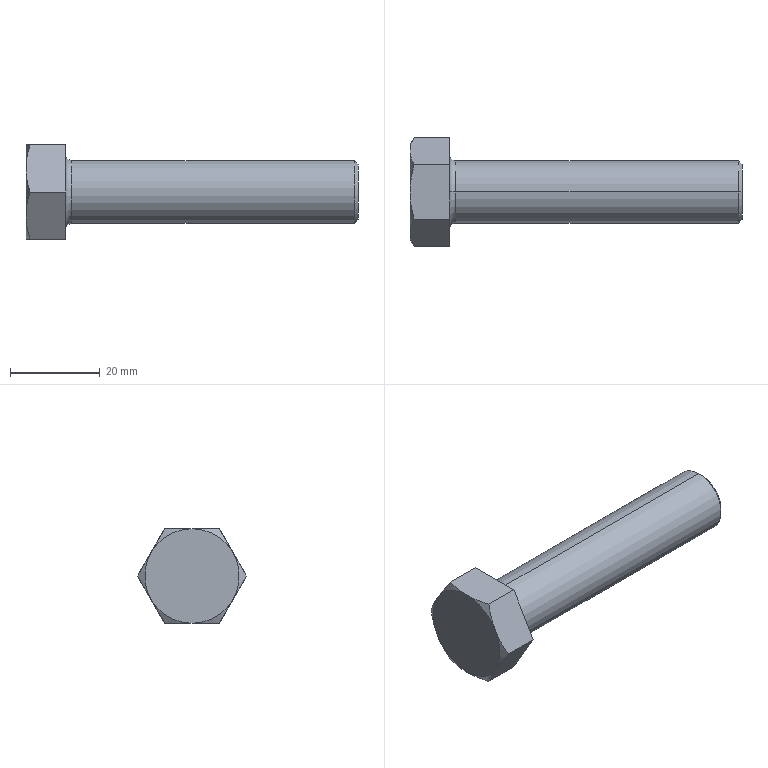Part | SolidWorks | features Chamfer 2, RevCut 2, Revolution 2, Extrusion 1, ICE 1 | 1 solid | 21 faces | box 73.8 x 24.249 x 21 mm | volume 13362 mm3 | plane 9 | cone 8 | cylinder 2 | torus 2 | commonest cylinder face diameters 14 x2
STEP:
#1=CARTESIAN_POINT('',(73.8,0.,-6.222));
#2=VERTEX_POINT('',#1);
#3=CARTESIAN_POINT('',(73.8,0.,6.222));
#4=VERTEX_POINT('',#3);
#5=CARTESIAN_POINT('',(73.8,0.,0.));
#6=DIRECTION('',(1.,0.,0.));
#7=DIRECTION('',(0.,0.,1.));
#8=AXIS2_PLACEMENT_3D('',#5,#6,#7);
#9=CIRCLE('',#8,6.222);
#10=EDGE_CURVE('',#2,#4,#9,.T.);
#11=ORIENTED_EDGE('',*,*,#10,.F.);
#12=CARTESIAN_POINT('',(73.022,0.,-7.));
#13=VERTEX_POINT('',#12);
#14=CARTESIAN_POINT('',(73.022,0.,-7.));
#15=DIRECTION('',(-0.7071,0.,-0.7071));
#16=VECTOR('',#15,1000.);
#17=LINE('',#14,#16);
#18=EDGE_CURVE('',#2,#13,#17,.T.);
#19=ORIENTED_EDGE('',*,*,#18,.T.);
#20=CARTESIAN_POINT('',(73.022,0.,7.));
#21=VERTEX_POINT('',#20);
#22=CARTESIAN_POINT('',(73.022,0.,0.));
#23=DIRECTION('',(-1.,0.,0.));
#24=DIRECTION('',(0.,0.,1.));
#25=AXIS2_PLACEMENT_3D('',#22,#23,#24);
#26=CIRCLE('',#25,7.);
#27=EDGE_CURVE('',#21,#13,#26,.T.);
#28=ORIENTED_EDGE('',*,*,#27,.F.);
#29=CARTESIAN_POINT('',(73.022,0.,7.));
#30=DIRECTION('',(-0.7071,0.,0.7071));
#31=VECTOR('',#30,1000.);
#32=LINE('',#29,#31);
#33=EDGE_CURVE('',#4,#21,#32,.T.);
#34=ORIENTED_EDGE('',*,*,#33,.F.);
#35=EDGE_LOOP('',(#11,#19,#28,#34));
#36=FACE_OUTER_BOUND('',#35,.T.);
#37=CARTESIAN_POINT('',(73.022,0.,0.));
#38=DIRECTION('',(-1.,0.,0.));
#39=DIRECTION('',(0.,0.,1.));
#40=AXIS2_PLACEMENT_3D('',#37,#38,#39);
#41=CONICAL_SURFACE('',#40,7.,0.7854);
#42=ADVANCED_FACE('',(#36),#41,.T.);
#43=ORIENTED_EDGE('',*,*,#27,.T.);
#44=CARTESIAN_POINT('',(10.15,0.,-7.));
#45=VERTEX_POINT('',#44);
#46=CARTESIAN_POINT('',(8.8,0.,-7.));
#47=DIRECTION('',(-1.,0.,0.));
#48=VECTOR('',#47,1000.);
#49=LINE('',#46,#48);
#50=EDGE_CURVE('',#13,#45,#49,.T.);
#51=ORIENTED_EDGE('',*,*,#50,.T.);
#52=CARTESIAN_POINT('',(10.15,0.,7.));
#53=VERTEX_POINT('',#52);
#54=CARTESIAN_POINT('',(10.15,0.,0.));
#55=DIRECTION('',(-1.,0.,0.));
#56=DIRECTION('',(0.,0.,1.));
#57=AXIS2_PLACEMENT_3D('',#54,#55,#56);
#58=CIRCLE('',#57,7.);
#59=EDGE_CURVE('',#53,#45,#58,.T.);
#60=ORIENTED_EDGE('',*,*,#59,.F.);
#61=CARTESIAN_POINT('',(8.8,0.,7.));
#62=DIRECTION('',(-1.,0.,0.));
#63=VECTOR('',#62,1000.);
#64=LINE('',#61,#63);
#65=EDGE_CURVE('',#21,#53,#64,.T.);
#66=ORIENTED_EDGE('',*,*,#65,.F.);
#67=EDGE_LOOP('',(#43,#51,#60,#66));
#68=FACE_OUTER_BOUND('',#67,.T.);
#69=CARTESIAN_POINT('',(8.8,0.,0.));
#70=DIRECTION('',(-1.,0.,0.));
#71=DIRECTION('',(0.,0.,1.));
#72=AXIS2_PLACEMENT_3D('',#69,#70,#71);
#73=CYLINDRICAL_SURFACE('',#72,7.);
#74=ADVANCED_FACE('',(#68),#73,.T.);
#75=CARTESIAN_POINT('',(8.8,0.,-8.35));
#76=VERTEX_POINT('',#75);
#77=CARTESIAN_POINT('',(8.8,0.,8.35));
#78=VERTEX_POINT('',#77);
#79=CARTESIAN_POINT('',(8.8,0.,0.));
#80=DIRECTION('',(-1.,0.,0.));
#81=DIRECTION('',(0.,0.,1.));
#82=AXIS2_PLACEMENT_3D('',#79,#80,#81);
#83=CIRCLE('',#82,8.35);
#84=EDGE_CURVE('',#76,#78,#83,.T.);
#85=ORIENTED_EDGE('',*,*,#84,.F.);
#86=CARTESIAN_POINT('',(10.15,0.,-8.35));
#87=DIRECTION('',(0.,1.,0.));
#88=DIRECTION('',(0.,0.,1.));
#89=AXIS2_PLACEMENT_3D('',#86,#87,#88);
#90=CIRCLE('',#89,1.35);
#91=EDGE_CURVE('',#76,#45,#90,.T.);
#92=ORIENTED_EDGE('',*,*,#91,.T.);
#93=CARTESIAN_POINT('',(10.15,0.,0.));
#94=DIRECTION('',(-1.,0.,0.));
#95=DIRECTION('',(0.,0.,1.));
#96=AXIS2_PLACEMENT_3D('',#93,#94,#95);
#97=CIRCLE('',#96,7.);
#98=EDGE_CURVE('',#45,#53,#97,.T.);
#99=ORIENTED_EDGE('',*,*,#98,.T.);
#100=CARTESIAN_POINT('',(10.15,0.,8.35));
#101=DIRECTION('',(0.,-1.,0.));
#102=DIRECTION('',(0.,0.,-1.));
#103=AXIS2_PLACEMENT_3D('',#100,#101,#102);
#104=CIRCLE('',#103,1.35);
#105=EDGE_CURVE('',#78,#53,#104,.T.);
#106=ORIENTED_EDGE('',*,*,#105,.F.);
#107=EDGE_LOOP('',(#85,#92,#99,#106));
#108=FACE_OUTER_BOUND('',#107,.T.);
#109=CARTESIAN_POINT('',(10.15,0.,0.));
#110=DIRECTION('',(-1.,0.,0.));
#111=DIRECTION('',(0.,0.,1.));
#112=AXIS2_PLACEMENT_3D('',#109,#110,#111);
#113=TOROIDAL_SURFACE('',#112,8.35,1.35);
#114=ADVANCED_FACE('',(#108),#113,.F.);
#115=CARTESIAN_POINT('',(8.8,-6.062,-10.5));
#116=VERTEX_POINT('',#115);
#117=CARTESIAN_POINT('',(8.8,6.062,-10.5));
#118=VERTEX_POINT('',#117);
#119=CARTESIAN_POINT('',(8.8,-6.062,-10.5));
#120=DIRECTION('',(0.,1.,0.));
#121=VECTOR('',#120,1000.);
#122=LINE('',#119,#121);
#123=EDGE_CURVE('',#116,#118,#122,.T.);
#124=ORIENTED_EDGE('',*,*,#123,.T.);
#125=CARTESIAN_POINT('',(8.8,12.124,0.));
#126=VERTEX_POINT('',#125);
#127=CARTESIAN_POINT('',(8.8,6.062,-10.5));
#128=DIRECTION('',(0.,0.5,0.866));
#129=VECTOR('',#128,1000.);
#130=LINE('',#127,#129);
#131=EDGE_CURVE('',#118,#126,#130,.T.);
#132=ORIENTED_EDGE('',*,*,#131,.T.);
#133=CARTESIAN_POINT('',(8.8,6.062,10.5));
#134=VERTEX_POINT('',#133);
#135=CARTESIAN_POINT('',(8.8,12.124,0.));
#136=DIRECTION('',(0.,-0.5,0.866));
#137=VECTOR('',#136,1000.);
#138=LINE('',#135,#137);
#139=EDGE_CURVE('',#126,#134,#138,.T.);
#140=ORIENTED_EDGE('',*,*,#139,.T.);
#141=CARTESIAN_POINT('',(8.8,-6.062,10.5));
#142=VERTEX_POINT('',#141);
#143=CARTESIAN_POINT('',(8.8,6.062,10.5));
#144=DIRECTION('',(0.,-1.,0.));
#145=VECTOR('',#144,1000.);
#146=LINE('',#143,#145);
#147=EDGE_CURVE('',#134,#142,#146,.T.);
#148=ORIENTED_EDGE('',*,*,#147,.T.);
#149=CARTESIAN_POINT('',(8.8,-12.124,0.));
#150=VERTEX_POINT('',#149);
#151=CARTESIAN_POINT('',(8.8,-6.062,10.5));
#152=DIRECTION('',(0.,-0.5,-0.866));
#153=VECTOR('',#152,1000.);
#154=LINE('',#151,#153);
#155=EDGE_CURVE('',#142,#150,#154,.T.);
#156=ORIENTED_EDGE('',*,*,#155,.T.);
#157=CARTESIAN_POINT('',(8.8,-12.124,0.));
#158=DIRECTION('',(0.,0.5,-0.866));
#159=VECTOR('',#158,1000.);
#160=LINE('',#157,#159);
#161=EDGE_CURVE('',#150,#116,#160,.T.);
#162=ORIENTED_EDGE('',*,*,#161,.T.);
#163=EDGE_LOOP('',(#124,#132,#140,#148,#156,#162));
#164=FACE_OUTER_BOUND('',#163,.T.);
#165=CARTESIAN_POINT('',(8.8,0.,0.));
#166=DIRECTION('',(-1.,0.,0.));
#167=DIRECTION('',(0.,0.,1.));
#168=AXIS2_PLACEMENT_3D('',#165,#166,#167);
#169=CIRCLE('',#168,8.35);
#170=EDGE_CURVE('',#78,#76,#169,.T.);
#171=ORIENTED_EDGE('',*,*,#170,.T.);
#172=ORIENTED_EDGE('',*,*,#84,.T.);
#173=EDGE_LOOP('',(#171,#172));
#174=FACE_BOUND('',#173,.T.);
#175=CARTESIAN_POINT('',(8.8,6.062,-10.5));
#176=DIRECTION('',(1.,0.,0.));
#177=DIRECTION('',(0.,0.,-1.));
#178=AXIS2_PLACEMENT_3D('',#175,#176,#177);
#179=PLANE('',#178);
#180=ADVANCED_FACE('',(#164,#174),#179,.T.);
#181=CARTESIAN_POINT('',(0.9378,6.062,-10.5));
#182=VERTEX_POINT('',#181);
#183=CARTESIAN_POINT('',(0.,0.,-10.5));
#184=VERTEX_POINT('',#183);
#185=CARTESIAN_POINT('',(0.9378,6.062,-10.5));
#186=CARTESIAN_POINT('',(0.6549,5.082,-10.5));
#187=CARTESIAN_POINT('',(0.4192,4.089,-10.5));
#188=CARTESIAN_POINT('',(0.1727,2.57,-10.5));
#189=CARTESIAN_POINT('',(0.1084,2.058,-10.5));
#190=CARTESIAN_POINT('',(0.02178,1.027,-10.5));
#191=CARTESIAN_POINT('',(0.,0.5125,-10.5));
#192=CARTESIAN_POINT('',(0.,0.,-10.5));
#193=B_SPLINE_CURVE_WITH_KNOTS('',3,(#185,#186,#187,#188,#189,#190,#191,#192),.UNSPECIFIED.,.F.,.F.,(4,2,2,4),(0.004417,0.007477,0.009008,0.01054),.UNSPECIFIED.);
#194=EDGE_CURVE('',#182,#184,#193,.T.);
#195=ORIENTED_EDGE('',*,*,#194,.F.);
#196=CARTESIAN_POINT('',(8.8,6.062,-10.5));
#197=DIRECTION('',(-1.,0.,0.));
#198=VECTOR('',#197,1000.);
#199=LINE('',#196,#198);
#200=EDGE_CURVE('',#118,#182,#199,.T.);
#201=ORIENTED_EDGE('',*,*,#200,.F.);
#202=ORIENTED_EDGE('',*,*,#123,.F.);
#203=CARTESIAN_POINT('',(0.9378,-6.062,-10.5));
#204=VERTEX_POINT('',#203);
#205=CARTESIAN_POINT('',(8.8,-6.062,-10.5));
#206=DIRECTION('',(-1.,0.,0.));
#207=VECTOR('',#206,1000.);
#208=LINE('',#205,#207);
#209=EDGE_CURVE('',#116,#204,#208,.T.);
#210=ORIENTED_EDGE('',*,*,#209,.T.);
#211=CARTESIAN_POINT('',(0.,0.,-10.5));
#212=CARTESIAN_POINT('',(0.,-1.024,-10.5));
#213=CARTESIAN_POINT('',(0.08806,-2.042,-10.5));
#214=CARTESIAN_POINT('',(0.4145,-4.066,-10.5));
#215=CARTESIAN_POINT('',(0.6532,-5.076,-10.5));
#216=CARTESIAN_POINT('',(0.9378,-6.062,-10.5));
#217=B_SPLINE_CURVE_WITH_KNOTS('',3,(#211,#212,#213,#214,#215,#216),.UNSPECIFIED.,.F.,.F.,(4,2,4),(0.01054,0.0136,0.01665),.UNSPECIFIED.);
#218=EDGE_CURVE('',#184,#204,#217,.T.);
#219=ORIENTED_EDGE('',*,*,#218,.F.);
#220=EDGE_LOOP('',(#195,#201,#202,#210,#219));
#221=FACE_OUTER_BOUND('',#220,.T.);
#222=CARTESIAN_POINT('',(8.8,-6.062,-10.5));
#223=DIRECTION('',(0.,0.,1.));
#224=DIRECTION('',(0.,-1.,0.));
#225=AXIS2_PLACEMENT_3D('',#222,#223,#224);
#226=PLANE('',#225);
#227=ADVANCED_FACE('',(#221),#226,.F.);
#228=CARTESIAN_POINT('',(0.9378,12.124,0.));
#229=VERTEX_POINT('',#228);
#230=CARTESIAN_POINT('',(0.,9.093,-5.25));
#231=VERTEX_POINT('',#230);
#232=CARTESIAN_POINT('',(0.9378,12.124,0.));
#233=CARTESIAN_POINT('',(0.6515,11.629,-0.8588));
#234=CARTESIAN_POINT('',(0.4157,11.129,-1.724));
#235=CARTESIAN_POINT('',(0.08938,10.12,-3.472));
#236=CARTESIAN_POINT('',(0.,9.61,-4.356));
#237=CARTESIAN_POINT('',(0.,9.093,-5.25));
#238=B_SPLINE_CURVE_WITH_KNOTS('',3,(#232,#233,#234,#235,#236,#237),.UNSPECIFIED.,.F.,.F.,(4,2,4),(0.000000238,0.003067,0.006134),.UNSPECIFIED.);
#239=EDGE_CURVE('',#229,#231,#238,.T.);
#240=ORIENTED_EDGE('',*,*,#239,.F.);
#241=CARTESIAN_POINT('',(8.8,12.124,0.));
#242=DIRECTION('',(-1.,0.,0.));
#243=VECTOR('',#242,1000.);
#244=LINE('',#241,#243);
#245=EDGE_CURVE('',#126,#229,#244,.T.);
#246=ORIENTED_EDGE('',*,*,#245,.F.);
#247=ORIENTED_EDGE('',*,*,#131,.F.);
#248=ORIENTED_EDGE('',*,*,#200,.T.);
#249=CARTESIAN_POINT('',(0.,9.093,-5.25));
#250=CARTESIAN_POINT('',(0.,8.836,-5.696));
#251=CARTESIAN_POINT('',(0.02217,8.578,-6.143));
#252=CARTESIAN_POINT('',(0.1079,8.066,-7.028));
#253=CARTESIAN_POINT('',(0.1715,7.813,-7.468));
#254=CARTESIAN_POINT('',(0.4165,7.056,-8.779));
#255=CARTESIAN_POINT('',(0.6523,6.557,-9.643));
#256=CARTESIAN_POINT('',(0.9378,6.062,-10.5));
#257=B_SPLINE_CURVE_WITH_KNOTS('',3,(#249,#250,#251,#252,#253,#254,#255,#256),.UNSPECIFIED.,.F.,.F.,(4,2,2,4),(0.006134,0.007662,0.00919,0.01225),.UNSPECIFIED.);
#258=EDGE_CURVE('',#231,#182,#257,.T.);
#259=ORIENTED_EDGE('',*,*,#258,.F.);
#260=EDGE_LOOP('',(#240,#246,#247,#248,#259));
#261=FACE_OUTER_BOUND('',#260,.T.);
#262=CARTESIAN_POINT('',(8.8,6.062,-10.5));
#263=DIRECTION('',(0.,-0.866,0.5));
#264=DIRECTION('',(0.,-0.5,-0.866));
#265=AXIS2_PLACEMENT_3D('',#262,#263,#264);
#266=PLANE('',#265);
#267=ADVANCED_FACE('',(#261),#266,.F.);
#268=CARTESIAN_POINT('',(0.9378,6.062,10.5));
#269=VERTEX_POINT('',#268);
#270=CARTESIAN_POINT('',(0.,9.093,5.25));
#271=VERTEX_POINT('',#270);
#272=CARTESIAN_POINT('',(0.9378,6.062,10.5));
#273=CARTESIAN_POINT('',(0.6515,6.558,9.641));
#274=CARTESIAN_POINT('',(0.4157,7.057,8.776));
#275=CARTESIAN_POINT('',(0.08938,8.067,7.028));
#276=CARTESIAN_POINT('',(0.,8.577,6.144));
#277=CARTESIAN_POINT('',(0.,9.093,5.25));
#278=B_SPLINE_CURVE_WITH_KNOTS('',3,(#272,#273,#274,#275,#276,#277),.UNSPECIFIED.,.F.,.F.,(4,2,4),(0.000000238,0.003067,0.006134),.UNSPECIFIED.);
#279=EDGE_CURVE('',#269,#271,#278,.T.);
#280=ORIENTED_EDGE('',*,*,#279,.F.);
#281=CARTESIAN_POINT('',(8.8,6.062,10.5));
#282=DIRECTION('',(-1.,0.,0.));
#283=VECTOR('',#282,1000.);
#284=LINE('',#281,#283);
#285=EDGE_CURVE('',#134,#269,#284,.T.);
#286=ORIENTED_EDGE('',*,*,#285,.F.);
#287=ORIENTED_EDGE('',*,*,#139,.F.);
#288=ORIENTED_EDGE('',*,*,#245,.T.);
#289=CARTESIAN_POINT('',(0.,9.093,5.25));
#290=CARTESIAN_POINT('',(0.,9.351,4.804));
#291=CARTESIAN_POINT('',(0.02217,9.609,4.357));
#292=CARTESIAN_POINT('',(0.1079,10.12,3.472));
#293=CARTESIAN_POINT('',(0.1715,10.374,3.032));
#294=CARTESIAN_POINT('',(0.4165,11.131,1.721));
#295=CARTESIAN_POINT('',(0.6523,11.63,0.8567));
#296=CARTESIAN_POINT('',(0.9378,12.124,0.));
#297=B_SPLINE_CURVE_WITH_KNOTS('',3,(#289,#290,#291,#292,#293,#294,#295,#296),.UNSPECIFIED.,.F.,.F.,(4,2,2,4),(0.006134,0.007662,0.00919,0.01225),.UNSPECIFIED.);
#298=EDGE_CURVE('',#271,#229,#297,.T.);
#299=ORIENTED_EDGE('',*,*,#298,.F.);
#300=EDGE_LOOP('',(#280,#286,#287,#288,#299));
#301=FACE_OUTER_BOUND('',#300,.T.);
#302=CARTESIAN_POINT('',(8.8,12.124,0.));
#303=DIRECTION('',(0.,-0.866,-0.5));
#304=DIRECTION('',(0.,0.5,-0.866));
#305=AXIS2_PLACEMENT_3D('',#302,#303,#304);
#306=PLANE('',#305);
#307=ADVANCED_FACE('',(#301),#306,.F.);
#308=CARTESIAN_POINT('',(0.9378,-6.062,10.5));
#309=VERTEX_POINT('',#308);
#310=CARTESIAN_POINT('',(0.,0.,10.5));
#311=VERTEX_POINT('',#310);
#312=CARTESIAN_POINT('',(0.9378,-6.062,10.5));
#313=CARTESIAN_POINT('',(0.6532,-5.076,10.5));
#314=CARTESIAN_POINT('',(0.4145,-4.066,10.5));
#315=CARTESIAN_POINT('',(0.08806,-2.042,10.5));
#316=CARTESIAN_POINT('',(0.,-1.024,10.5));
#317=CARTESIAN_POINT('',(0.,0.,10.5));
#318=B_SPLINE_CURVE_WITH_KNOTS('',3,(#312,#313,#314,#315,#316,#317),.UNSPECIFIED.,.F.,.F.,(4,2,4),(0.01084,0.01391,0.01697),.UNSPECIFIED.);
#319=EDGE_CURVE('',#309,#311,#318,.T.);
#320=ORIENTED_EDGE('',*,*,#319,.F.);
#321=CARTESIAN_POINT('',(8.8,-6.062,10.5));
#322=DIRECTION('',(-1.,0.,0.));
#323=VECTOR('',#322,1000.);
#324=LINE('',#321,#323);
#325=EDGE_CURVE('',#142,#309,#324,.T.);
#326=ORIENTED_EDGE('',*,*,#325,.F.);
#327=ORIENTED_EDGE('',*,*,#147,.F.);
#328=ORIENTED_EDGE('',*,*,#285,.T.);
#329=CARTESIAN_POINT('',(0.,0.,10.5));
#330=CARTESIAN_POINT('',(0.,0.5125,10.5));
#331=CARTESIAN_POINT('',(0.02178,1.027,10.5));
#332=CARTESIAN_POINT('',(0.1084,2.058,10.5));
#333=CARTESIAN_POINT('',(0.1727,2.57,10.5));
#334=CARTESIAN_POINT('',(0.4192,4.089,10.5));
#335=CARTESIAN_POINT('',(0.6549,5.082,10.5));
#336=CARTESIAN_POINT('',(0.9378,6.062,10.5));
#337=B_SPLINE_CURVE_WITH_KNOTS('',3,(#329,#330,#331,#332,#333,#334,#335,#336),.UNSPECIFIED.,.F.,.F.,(4,2,2,4),(0.01697,0.01851,0.02004,0.02311),.UNSPECIFIED.);
#338=EDGE_CURVE('',#311,#269,#337,.T.);
#339=ORIENTED_EDGE('',*,*,#338,.F.);
#340=EDGE_LOOP('',(#320,#326,#327,#328,#339));
#341=FACE_OUTER_BOUND('',#340,.T.);
#342=CARTESIAN_POINT('',(8.8,6.062,10.5));
#343=DIRECTION('',(0.,0.,-1.));
#344=DIRECTION('',(-1.,0.,0.));
#345=AXIS2_PLACEMENT_3D('',#342,#343,#344);
#346=PLANE('',#345);
#347=ADVANCED_FACE('',(#341),#346,.F.);
#348=CARTESIAN_POINT('',(0.9378,-12.124,0.));
#349=VERTEX_POINT('',#348);
#350=CARTESIAN_POINT('',(0.,-9.093,5.25));
#351=VERTEX_POINT('',#350);
#352=CARTESIAN_POINT('',(0.9378,-12.124,0.));
#353=CARTESIAN_POINT('',(0.6515,-11.629,0.8588));
#354=CARTESIAN_POINT('',(0.4157,-11.129,1.724));
#355=CARTESIAN_POINT('',(0.08938,-10.12,3.472));
#356=CARTESIAN_POINT('',(0.,-9.61,4.356));
#357=CARTESIAN_POINT('',(0.,-9.093,5.25));
#358=B_SPLINE_CURVE_WITH_KNOTS('',3,(#352,#353,#354,#355,#356,#357),.UNSPECIFIED.,.F.,.F.,(4,2,4),(0.000000238,0.003067,0.006134),.UNSPECIFIED.);
#359=EDGE_CURVE('',#349,#351,#358,.T.);
#360=ORIENTED_EDGE('',*,*,#359,.F.);
#361=CARTESIAN_POINT('',(8.8,-12.124,0.));
#362=DIRECTION('',(-1.,0.,0.));
#363=VECTOR('',#362,1000.);
#364=LINE('',#361,#363);
#365=EDGE_CURVE('',#150,#349,#364,.T.);
#366=ORIENTED_EDGE('',*,*,#365,.F.);
#367=ORIENTED_EDGE('',*,*,#155,.F.);
#368=ORIENTED_EDGE('',*,*,#325,.T.);
#369=CARTESIAN_POINT('',(0.,-9.093,5.25));
#370=CARTESIAN_POINT('',(0.,-8.836,5.696));
#371=CARTESIAN_POINT('',(0.02217,-8.578,6.143));
#372=CARTESIAN_POINT('',(0.1079,-8.066,7.028));
#373=CARTESIAN_POINT('',(0.1715,-7.813,7.468));
#374=CARTESIAN_POINT('',(0.4165,-7.056,8.779));
#375=CARTESIAN_POINT('',(0.6523,-6.557,9.643));
#376=CARTESIAN_POINT('',(0.9378,-6.062,10.5));
#377=B_SPLINE_CURVE_WITH_KNOTS('',3,(#369,#370,#371,#372,#373,#374,#375,#376),.UNSPECIFIED.,.F.,.F.,(4,2,2,4),(0.006134,0.007662,0.00919,0.01225),.UNSPECIFIED.);
#378=EDGE_CURVE('',#351,#309,#377,.T.);
#379=ORIENTED_EDGE('',*,*,#378,.F.);
#380=EDGE_LOOP('',(#360,#366,#367,#368,#379));
#381=FACE_OUTER_BOUND('',#380,.T.);
#382=CARTESIAN_POINT('',(8.8,-6.062,10.5));
#383=DIRECTION('',(0.,0.866,-0.5));
#384=DIRECTION('',(0.,0.5,0.866));
#385=AXIS2_PLACEMENT_3D('',#382,#383,#384);
#386=PLANE('',#385);
#387=ADVANCED_FACE('',(#381),#386,.F.);
#388=CARTESIAN_POINT('',(0.,-9.093,-5.25));
#389=VERTEX_POINT('',#388);
#390=CARTESIAN_POINT('',(0.9378,-6.062,-10.5));
#391=CARTESIAN_POINT('',(0.6515,-6.558,-9.641));
#392=CARTESIAN_POINT('',(0.4157,-7.057,-8.776));
#393=CARTESIAN_POINT('',(0.08938,-8.067,-7.028));
#394=CARTESIAN_POINT('',(0.,-8.577,-6.144));
#395=CARTESIAN_POINT('',(0.,-9.093,-5.25));
#396=B_SPLINE_CURVE_WITH_KNOTS('',3,(#390,#391,#392,#393,#394,#395),.UNSPECIFIED.,.F.,.F.,(4,2,4),(0.000000238,0.003067,0.006134),.UNSPECIFIED.);
#397=EDGE_CURVE('',#204,#389,#396,.T.);
#398=ORIENTED_EDGE('',*,*,#397,.F.);
#399=ORIENTED_EDGE('',*,*,#209,.F.);
#400=ORIENTED_EDGE('',*,*,#161,.F.);
#401=ORIENTED_EDGE('',*,*,#365,.T.);
#402=CARTESIAN_POINT('',(0.,-9.093,-5.25));
#403=CARTESIAN_POINT('',(0.,-9.351,-4.804));
#404=CARTESIAN_POINT('',(0.02217,-9.609,-4.357));
#405=CARTESIAN_POINT('',(0.1079,-10.12,-3.472));
#406=CARTESIAN_POINT('',(0.1715,-10.374,-3.032));
#407=CARTESIAN_POINT('',(0.4165,-11.131,-1.721));
#408=CARTESIAN_POINT('',(0.6523,-11.63,-0.8567));
#409=CARTESIAN_POINT('',(0.9378,-12.124,0.));
#410=B_SPLINE_CURVE_WITH_KNOTS('',3,(#402,#403,#404,#405,#406,#407,#408,#409),.UNSPECIFIED.,.F.,.F.,(4,2,2,4),(0.006134,0.007662,0.00919,0.01225),.UNSPECIFIED.);
#411=EDGE_CURVE('',#389,#349,#410,.T.);
#412=ORIENTED_EDGE('',*,*,#411,.F.);
#413=EDGE_LOOP('',(#398,#399,#400,#401,#412));
#414=FACE_OUTER_BOUND('',#413,.T.);
#415=CARTESIAN_POINT('',(8.8,-12.124,0.));
#416=DIRECTION('',(0.,0.866,0.5));
#417=DIRECTION('',(0.,-0.5,0.866));
#418=AXIS2_PLACEMENT_3D('',#415,#416,#417);
#419=PLANE('',#418);
#420=ADVANCED_FACE('',(#414),#419,.F.);
#421=ORIENTED_EDGE('',*,*,#218,.T.);
#422=ORIENTED_EDGE('',*,*,#397,.T.);
#423=CARTESIAN_POINT('',(0.,0.,0.));
#424=DIRECTION('',(1.,0.,0.));
#425=DIRECTION('',(0.,0.,-1.));
#426=AXIS2_PLACEMENT_3D('',#423,#424,#425);
#427=CIRCLE('',#426,10.5);
#428=EDGE_CURVE('',#389,#184,#427,.T.);
#429=ORIENTED_EDGE('',*,*,#428,.T.);
#430=EDGE_LOOP('',(#421,#422,#429));
#431=FACE_OUTER_BOUND('',#430,.T.);
#432=CARTESIAN_POINT('',(0.,0.,0.));
#433=DIRECTION('',(1.,0.,0.));
#434=DIRECTION('',(0.,0.,1.));
#435=AXIS2_PLACEMENT_3D('',#432,#433,#434);
#436=CONICAL_SURFACE('',#435,10.5,1.047);
#437=ADVANCED_FACE('',(#431),#436,.T.);
#438=ORIENTED_EDGE('',*,*,#359,.T.);
#439=CARTESIAN_POINT('',(0.,0.,0.));
#440=DIRECTION('',(1.,0.,0.));
#441=DIRECTION('',(0.,0.,-1.));
#442=AXIS2_PLACEMENT_3D('',#439,#440,#441);
#443=CIRCLE('',#442,10.5);
#444=EDGE_CURVE('',#351,#389,#443,.T.);
#445=ORIENTED_EDGE('',*,*,#444,.T.);
#446=ORIENTED_EDGE('',*,*,#411,.T.);
#447=EDGE_LOOP('',(#438,#445,#446));
#448=FACE_OUTER_BOUND('',#447,.T.);
#449=CARTESIAN_POINT('',(0.,0.,0.));
#450=DIRECTION('',(1.,0.,0.));
#451=DIRECTION('',(0.,0.,1.));
#452=AXIS2_PLACEMENT_3D('',#449,#450,#451);
#453=CONICAL_SURFACE('',#452,10.5,1.047);
#454=ADVANCED_FACE('',(#448),#453,.T.);
#455=ORIENTED_EDGE('',*,*,#319,.T.);
#456=CARTESIAN_POINT('',(0.,0.,0.));
#457=DIRECTION('',(1.,0.,0.));
#458=DIRECTION('',(0.,0.,-1.));
#459=AXIS2_PLACEMENT_3D('',#456,#457,#458);
#460=CIRCLE('',#459,10.5);
#461=EDGE_CURVE('',#311,#351,#460,.T.);
#462=ORIENTED_EDGE('',*,*,#461,.T.);
#463=ORIENTED_EDGE('',*,*,#378,.T.);
#464=EDGE_LOOP('',(#455,#462,#463));
#465=FACE_OUTER_BOUND('',#464,.T.);
#466=CARTESIAN_POINT('',(0.,0.,0.));
#467=DIRECTION('',(1.,0.,0.));
#468=DIRECTION('',(0.,0.,1.));
#469=AXIS2_PLACEMENT_3D('',#466,#467,#468);
#470=CONICAL_SURFACE('',#469,10.5,1.047);
#471=ADVANCED_FACE('',(#465),#470,.T.);
#472=ORIENTED_EDGE('',*,*,#279,.T.);
#473=CARTESIAN_POINT('',(0.,0.,0.));
#474=DIRECTION('',(-1.,0.,0.));
#475=DIRECTION('',(0.,0.,1.));
#476=AXIS2_PLACEMENT_3D('',#473,#474,#475);
#477=CIRCLE('',#476,10.5);
#478=EDGE_CURVE('',#311,#271,#477,.T.);
#479=ORIENTED_EDGE('',*,*,#478,.F.);
#480=ORIENTED_EDGE('',*,*,#338,.T.);
#481=EDGE_LOOP('',(#472,#479,#480));
#482=FACE_OUTER_BOUND('',#481,.T.);
#483=CARTESIAN_POINT('',(0.,0.,0.));
#484=DIRECTION('',(1.,0.,0.));
#485=DIRECTION('',(0.,0.,1.));
#486=AXIS2_PLACEMENT_3D('',#483,#484,#485);
#487=CONICAL_SURFACE('',#486,10.5,1.047);
#488=ADVANCED_FACE('',(#482),#487,.T.);
#489=ORIENTED_EDGE('',*,*,#298,.T.);
#490=ORIENTED_EDGE('',*,*,#239,.T.);
#491=CARTESIAN_POINT('',(0.,0.,0.));
#492=DIRECTION('',(1.,0.,0.));
#493=DIRECTION('',(0.,0.,-1.));
#494=AXIS2_PLACEMENT_3D('',#491,#492,#493);
#495=CIRCLE('',#494,10.5);
#496=EDGE_CURVE('',#231,#271,#495,.T.);
#497=ORIENTED_EDGE('',*,*,#496,.T.);
#498=EDGE_LOOP('',(#489,#490,#497));
#499=FACE_OUTER_BOUND('',#498,.T.);
#500=CARTESIAN_POINT('',(0.,0.,0.));
#501=DIRECTION('',(1.,0.,0.));
#502=DIRECTION('',(0.,0.,1.));
#503=AXIS2_PLACEMENT_3D('',#500,#501,#502);
#504=CONICAL_SURFACE('',#503,10.5,1.047);
#505=ADVANCED_FACE('',(#499),#504,.T.);
#506=ORIENTED_EDGE('',*,*,#258,.T.);
#507=ORIENTED_EDGE('',*,*,#194,.T.);
#508=CARTESIAN_POINT('',(0.,0.,0.));
#509=DIRECTION('',(1.,0.,0.));
#510=DIRECTION('',(0.,0.,-1.));
#511=AXIS2_PLACEMENT_3D('',#508,#509,#510);
#512=CIRCLE('',#511,10.5);
#513=EDGE_CURVE('',#184,#231,#512,.T.);
#514=ORIENTED_EDGE('',*,*,#513,.T.);
#515=EDGE_LOOP('',(#506,#507,#514));
#516=FACE_OUTER_BOUND('',#515,.T.);
#517=CARTESIAN_POINT('',(0.,0.,0.));
#518=DIRECTION('',(1.,0.,0.));
#519=DIRECTION('',(0.,0.,1.));
#520=AXIS2_PLACEMENT_3D('',#517,#518,#519);
#521=CONICAL_SURFACE('',#520,10.5,1.047);
#522=ADVANCED_FACE('',(#516),#521,.T.);
#523=ORIENTED_EDGE('',*,*,#513,.F.);
#524=ORIENTED_EDGE('',*,*,#428,.F.);
#525=ORIENTED_EDGE('',*,*,#444,.F.);
#526=ORIENTED_EDGE('',*,*,#461,.F.);
#527=ORIENTED_EDGE('',*,*,#478,.T.);
#528=ORIENTED_EDGE('',*,*,#496,.F.);
#529=EDGE_LOOP('',(#523,#524,#525,#526,#527,#528));
#530=FACE_OUTER_BOUND('',#529,.T.);
#531=CARTESIAN_POINT('',(0.,6.062,-10.5));
#532=DIRECTION('',(1.,0.,0.));
#533=DIRECTION('',(0.,0.,-1.));
#534=AXIS2_PLACEMENT_3D('',#531,#532,#533);
#535=PLANE('',#534);
#536=ADVANCED_FACE('',(#530),#535,.F.);
#537=ORIENTED_EDGE('',*,*,#91,.F.);
#538=ORIENTED_EDGE('',*,*,#170,.F.);
#539=ORIENTED_EDGE('',*,*,#105,.T.);
#540=ORIENTED_EDGE('',*,*,#59,.T.);
#541=EDGE_LOOP('',(#537,#538,#539,#540));
#542=FACE_OUTER_BOUND('',#541,.T.);
#543=CARTESIAN_POINT('',(10.15,0.,0.));
#544=DIRECTION('',(-1.,0.,0.));
#545=DIRECTION('',(0.,0.,1.));
#546=AXIS2_PLACEMENT_3D('',#543,#544,#545);
#547=TOROIDAL_SURFACE('',#546,8.35,1.35);
#548=ADVANCED_FACE('',(#542),#547,.F.);
#549=CARTESIAN_POINT('',(73.8,0.,0.));
#550=DIRECTION('',(1.,0.,0.));
#551=DIRECTION('',(0.,0.,1.));
#552=AXIS2_PLACEMENT_3D('',#549,#550,#551);
#553=CIRCLE('',#552,6.222);
#554=EDGE_CURVE('',#4,#2,#553,.T.);
#555=ORIENTED_EDGE('',*,*,#554,.T.);
#556=ORIENTED_EDGE('',*,*,#10,.T.);
#557=EDGE_LOOP('',(#555,#556));
#558=FACE_OUTER_BOUND('',#557,.T.);
#559=CARTESIAN_POINT('',(73.8,7.,0.));
#560=DIRECTION('',(-1.,0.,0.));
#561=DIRECTION('',(0.,0.,1.));
#562=AXIS2_PLACEMENT_3D('',#559,#560,#561);
#563=PLANE('',#562);
#564=ADVANCED_FACE('',(#558),#563,.F.);
#565=ORIENTED_EDGE('',*,*,#50,.F.);
#566=CARTESIAN_POINT('',(73.022,0.,0.));
#567=DIRECTION('',(-1.,0.,0.));
#568=DIRECTION('',(0.,0.,1.));
#569=AXIS2_PLACEMENT_3D('',#566,#567,#568);
#570=CIRCLE('',#569,7.);
#571=EDGE_CURVE('',#13,#21,#570,.T.);
#572=ORIENTED_EDGE('',*,*,#571,.T.);
#573=ORIENTED_EDGE('',*,*,#65,.T.);
#574=ORIENTED_EDGE('',*,*,#98,.F.);
#575=EDGE_LOOP('',(#565,#572,#573,#574));
#576=FACE_OUTER_BOUND('',#575,.T.);
#577=CARTESIAN_POINT('',(8.8,0.,0.));
#578=DIRECTION('',(-1.,0.,0.));
#579=DIRECTION('',(0.,0.,1.));
#580=AXIS2_PLACEMENT_3D('',#577,#578,#579);
#581=CYLINDRICAL_SURFACE('',#580,7.);
#582=ADVANCED_FACE('',(#576),#581,.T.);
#583=ORIENTED_EDGE('',*,*,#18,.F.);
#584=ORIENTED_EDGE('',*,*,#554,.F.);
#585=ORIENTED_EDGE('',*,*,#33,.T.);
#586=ORIENTED_EDGE('',*,*,#571,.F.);
#587=EDGE_LOOP('',(#583,#584,#585,#586));
#588=FACE_OUTER_BOUND('',#587,.T.);
#589=CARTESIAN_POINT('',(73.022,0.,0.));
#590=DIRECTION('',(-1.,0.,0.));
#591=DIRECTION('',(0.,0.,1.));
#592=AXIS2_PLACEMENT_3D('',#589,#590,#591);
#593=CONICAL_SURFACE('',#592,7.,0.7854);
#594=ADVANCED_FACE('',(#588),#593,.T.);
#595=CLOSED_SHELL('',(#42,#74,#114,#180,#227,#267,#307,#347,#387,#420,#437,#454,#471,#488,#505,#522,#536,#548,#564,#582,#594));
#596=MANIFOLD_SOLID_BREP('',#595);
#597=CARTESIAN_POINT('',(0.,0.,0.));
#598=DIRECTION('',(0.,0.,1.));
#599=DIRECTION('',(1.,0.,0.));
#600=AXIS2_PLACEMENT_3D('',#597,#598,#599);
#601=(LENGTH_UNIT()NAMED_UNIT(*)SI_UNIT(.MILLI.,.METRE.));
#602=UNCERTAINTY_MEASURE_WITH_UNIT(LENGTH_MEASURE(0.00001),#601,'','');
#603=(NAMED_UNIT(*)PLANE_ANGLE_UNIT()SI_UNIT($,.RADIAN.));
#604=(NAMED_UNIT(*)SI_UNIT($,.STERADIAN.)SOLID_ANGLE_UNIT());
#605=(GEOMETRIC_REPRESENTATION_CONTEXT(3)GLOBAL_UNCERTAINTY_ASSIGNED_CONTEXT((#602))GLOBAL_UNIT_ASSIGNED_CONTEXT((#601,#603,#604))REPRESENTATION_CONTEXT('',''));
#606=ADVANCED_BREP_SHAPE_REPRESENTATION('',(#596,#600),#605);